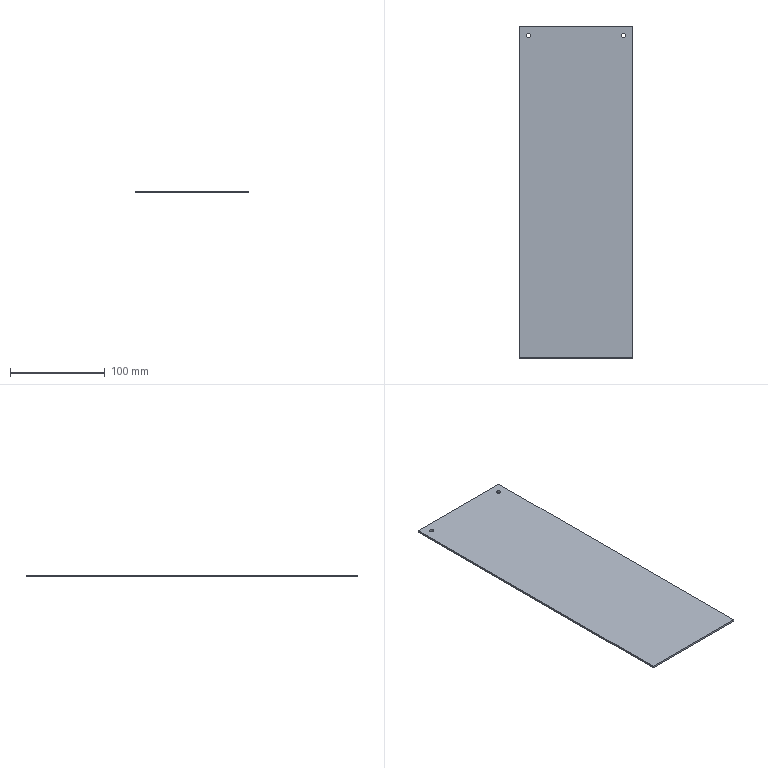Part | SolidWorks | features Extrusion 1, ICE 1 | 1 solid | 10 faces | box 120 x 350 x 2 mm | volume 83936 mm3 | plane 6 | cylinder 4 | commonest cylinder face diameters 4.5 x4
STEP:
#1=CARTESIAN_POINT('',(47.75,165.,0.));
#2=VERTEX_POINT('',#1);
#3=CARTESIAN_POINT('',(52.25,165.,0.));
#4=VERTEX_POINT('',#3);
#5=CARTESIAN_POINT('',(50.,165.,0.));
#6=DIRECTION('',(0.,0.,1.));
#7=DIRECTION('',(1.,0.,0.));
#8=AXIS2_PLACEMENT_3D('',#5,#6,#7);
#9=CIRCLE('',#8,2.25);
#10=EDGE_CURVE('',#2,#4,#9,.T.);
#11=ORIENTED_EDGE('',*,*,#10,.F.);
#12=CARTESIAN_POINT('',(47.75,165.,2.));
#13=VERTEX_POINT('',#12);
#14=CARTESIAN_POINT('',(47.75,165.,-8.));
#15=DIRECTION('',(0.,0.,1.));
#16=VECTOR('',#15,1000.);
#17=LINE('',#14,#16);
#18=EDGE_CURVE('',#2,#13,#17,.T.);
#19=ORIENTED_EDGE('',*,*,#18,.T.);
#20=CARTESIAN_POINT('',(52.25,165.,2.));
#21=VERTEX_POINT('',#20);
#22=CARTESIAN_POINT('',(50.,165.,2.));
#23=DIRECTION('',(0.,0.,1.));
#24=DIRECTION('',(1.,0.,0.));
#25=AXIS2_PLACEMENT_3D('',#22,#23,#24);
#26=CIRCLE('',#25,2.25);
#27=EDGE_CURVE('',#13,#21,#26,.T.);
#28=ORIENTED_EDGE('',*,*,#27,.T.);
#29=CARTESIAN_POINT('',(52.25,165.,-8.));
#30=DIRECTION('',(0.,0.,1.));
#31=VECTOR('',#30,1000.);
#32=LINE('',#29,#31);
#33=EDGE_CURVE('',#4,#21,#32,.T.);
#34=ORIENTED_EDGE('',*,*,#33,.F.);
#35=EDGE_LOOP('',(#11,#19,#28,#34));
#36=FACE_OUTER_BOUND('',#35,.T.);
#37=CARTESIAN_POINT('',(50.,165.,-8.));
#38=DIRECTION('',(0.,0.,1.));
#39=DIRECTION('',(1.,0.,0.));
#40=AXIS2_PLACEMENT_3D('',#37,#38,#39);
#41=CYLINDRICAL_SURFACE('',#40,2.25);
#42=ADVANCED_FACE('',(#36),#41,.F.);
#43=CARTESIAN_POINT('',(-52.25,165.,0.));
#44=VERTEX_POINT('',#43);
#45=CARTESIAN_POINT('',(-47.75,165.,0.));
#46=VERTEX_POINT('',#45);
#47=CARTESIAN_POINT('',(-50.,165.,0.));
#48=DIRECTION('',(0.,0.,1.));
#49=DIRECTION('',(1.,0.,0.));
#50=AXIS2_PLACEMENT_3D('',#47,#48,#49);
#51=CIRCLE('',#50,2.25);
#52=EDGE_CURVE('',#44,#46,#51,.T.);
#53=ORIENTED_EDGE('',*,*,#52,.F.);
#54=CARTESIAN_POINT('',(-52.25,165.,2.));
#55=VERTEX_POINT('',#54);
#56=CARTESIAN_POINT('',(-52.25,165.,-8.));
#57=DIRECTION('',(0.,0.,1.));
#58=VECTOR('',#57,1000.);
#59=LINE('',#56,#58);
#60=EDGE_CURVE('',#44,#55,#59,.T.);
#61=ORIENTED_EDGE('',*,*,#60,.T.);
#62=CARTESIAN_POINT('',(-47.75,165.,2.));
#63=VERTEX_POINT('',#62);
#64=CARTESIAN_POINT('',(-50.,165.,2.));
#65=DIRECTION('',(0.,0.,1.));
#66=DIRECTION('',(1.,0.,0.));
#67=AXIS2_PLACEMENT_3D('',#64,#65,#66);
#68=CIRCLE('',#67,2.25);
#69=EDGE_CURVE('',#55,#63,#68,.T.);
#70=ORIENTED_EDGE('',*,*,#69,.T.);
#71=CARTESIAN_POINT('',(-47.75,165.,-8.));
#72=DIRECTION('',(0.,0.,1.));
#73=VECTOR('',#72,1000.);
#74=LINE('',#71,#73);
#75=EDGE_CURVE('',#46,#63,#74,.T.);
#76=ORIENTED_EDGE('',*,*,#75,.F.);
#77=EDGE_LOOP('',(#53,#61,#70,#76));
#78=FACE_OUTER_BOUND('',#77,.T.);
#79=CARTESIAN_POINT('',(-50.,165.,-8.));
#80=DIRECTION('',(0.,0.,1.));
#81=DIRECTION('',(1.,0.,0.));
#82=AXIS2_PLACEMENT_3D('',#79,#80,#81);
#83=CYLINDRICAL_SURFACE('',#82,2.25);
#84=ADVANCED_FACE('',(#78),#83,.F.);
#85=CARTESIAN_POINT('',(60.,-175.,0.));
#86=VERTEX_POINT('',#85);
#87=CARTESIAN_POINT('',(60.,175.,0.));
#88=VERTEX_POINT('',#87);
#89=CARTESIAN_POINT('',(60.,175.,0.));
#90=DIRECTION('',(0.,1.,0.));
#91=VECTOR('',#90,1000.);
#92=LINE('',#89,#91);
#93=EDGE_CURVE('',#86,#88,#92,.T.);
#94=ORIENTED_EDGE('',*,*,#93,.T.);
#95=CARTESIAN_POINT('',(60.,175.,2.));
#96=VERTEX_POINT('',#95);
#97=CARTESIAN_POINT('',(60.,175.,2.));
#98=DIRECTION('',(0.,0.,-1.));
#99=VECTOR('',#98,1000.);
#100=LINE('',#97,#99);
#101=EDGE_CURVE('',#96,#88,#100,.T.);
#102=ORIENTED_EDGE('',*,*,#101,.F.);
#103=CARTESIAN_POINT('',(60.,-175.,2.));
#104=VERTEX_POINT('',#103);
#105=CARTESIAN_POINT('',(60.,175.,2.));
#106=DIRECTION('',(0.,1.,0.));
#107=VECTOR('',#106,1000.);
#108=LINE('',#105,#107);
#109=EDGE_CURVE('',#104,#96,#108,.T.);
#110=ORIENTED_EDGE('',*,*,#109,.F.);
#111=CARTESIAN_POINT('',(60.,-175.,2.));
#112=DIRECTION('',(0.,0.,-1.));
#113=VECTOR('',#112,1000.);
#114=LINE('',#111,#113);
#115=EDGE_CURVE('',#104,#86,#114,.T.);
#116=ORIENTED_EDGE('',*,*,#115,.T.);
#117=EDGE_LOOP('',(#94,#102,#110,#116));
#118=FACE_OUTER_BOUND('',#117,.T.);
#119=CARTESIAN_POINT('',(60.,175.,2.));
#120=DIRECTION('',(-1.,0.,0.));
#121=DIRECTION('',(0.,0.,1.));
#122=AXIS2_PLACEMENT_3D('',#119,#120,#121);
#123=PLANE('',#122);
#124=ADVANCED_FACE('',(#118),#123,.F.);
#125=CARTESIAN_POINT('',(-60.,175.,0.));
#126=VERTEX_POINT('',#125);
#127=CARTESIAN_POINT('',(-60.,175.,0.));
#128=DIRECTION('',(-1.,0.,0.));
#129=VECTOR('',#128,1000.);
#130=LINE('',#127,#129);
#131=EDGE_CURVE('',#88,#126,#130,.T.);
#132=ORIENTED_EDGE('',*,*,#131,.T.);
#133=CARTESIAN_POINT('',(-60.,175.,2.));
#134=VERTEX_POINT('',#133);
#135=CARTESIAN_POINT('',(-60.,175.,2.));
#136=DIRECTION('',(0.,0.,-1.));
#137=VECTOR('',#136,1000.);
#138=LINE('',#135,#137);
#139=EDGE_CURVE('',#134,#126,#138,.T.);
#140=ORIENTED_EDGE('',*,*,#139,.F.);
#141=CARTESIAN_POINT('',(-60.,175.,2.));
#142=DIRECTION('',(-1.,0.,0.));
#143=VECTOR('',#142,1000.);
#144=LINE('',#141,#143);
#145=EDGE_CURVE('',#96,#134,#144,.T.);
#146=ORIENTED_EDGE('',*,*,#145,.F.);
#147=ORIENTED_EDGE('',*,*,#101,.T.);
#148=EDGE_LOOP('',(#132,#140,#146,#147));
#149=FACE_OUTER_BOUND('',#148,.T.);
#150=CARTESIAN_POINT('',(-60.,175.,2.));
#151=DIRECTION('',(0.,-1.,0.));
#152=DIRECTION('',(0.,0.,-1.));
#153=AXIS2_PLACEMENT_3D('',#150,#151,#152);
#154=PLANE('',#153);
#155=ADVANCED_FACE('',(#149),#154,.F.);
#156=CARTESIAN_POINT('',(-60.,-175.,0.));
#157=VERTEX_POINT('',#156);
#158=CARTESIAN_POINT('',(-60.,175.,0.));
#159=DIRECTION('',(0.,-1.,0.));
#160=VECTOR('',#159,1000.);
#161=LINE('',#158,#160);
#162=EDGE_CURVE('',#126,#157,#161,.T.);
#163=ORIENTED_EDGE('',*,*,#162,.T.);
#164=CARTESIAN_POINT('',(-60.,-175.,2.));
#165=VERTEX_POINT('',#164);
#166=CARTESIAN_POINT('',(-60.,-175.,2.));
#167=DIRECTION('',(0.,0.,-1.));
#168=VECTOR('',#167,1000.);
#169=LINE('',#166,#168);
#170=EDGE_CURVE('',#165,#157,#169,.T.);
#171=ORIENTED_EDGE('',*,*,#170,.F.);
#172=CARTESIAN_POINT('',(-60.,175.,2.));
#173=DIRECTION('',(0.,-1.,0.));
#174=VECTOR('',#173,1000.);
#175=LINE('',#172,#174);
#176=EDGE_CURVE('',#134,#165,#175,.T.);
#177=ORIENTED_EDGE('',*,*,#176,.F.);
#178=ORIENTED_EDGE('',*,*,#139,.T.);
#179=EDGE_LOOP('',(#163,#171,#177,#178));
#180=FACE_OUTER_BOUND('',#179,.T.);
#181=CARTESIAN_POINT('',(-60.,175.,2.));
#182=DIRECTION('',(1.,0.,0.));
#183=DIRECTION('',(0.,0.,-1.));
#184=AXIS2_PLACEMENT_3D('',#181,#182,#183);
#185=PLANE('',#184);
#186=ADVANCED_FACE('',(#180),#185,.F.);
#187=CARTESIAN_POINT('',(-60.,-175.,0.));
#188=DIRECTION('',(1.,0.,0.));
#189=VECTOR('',#188,1000.);
#190=LINE('',#187,#189);
#191=EDGE_CURVE('',#157,#86,#190,.T.);
#192=ORIENTED_EDGE('',*,*,#191,.T.);
#193=ORIENTED_EDGE('',*,*,#115,.F.);
#194=CARTESIAN_POINT('',(-60.,-175.,2.));
#195=DIRECTION('',(1.,0.,0.));
#196=VECTOR('',#195,1000.);
#197=LINE('',#194,#196);
#198=EDGE_CURVE('',#165,#104,#197,.T.);
#199=ORIENTED_EDGE('',*,*,#198,.F.);
#200=ORIENTED_EDGE('',*,*,#170,.T.);
#201=EDGE_LOOP('',(#192,#193,#199,#200));
#202=FACE_OUTER_BOUND('',#201,.T.);
#203=CARTESIAN_POINT('',(-60.,-175.,2.));
#204=DIRECTION('',(0.,1.,0.));
#205=DIRECTION('',(0.,0.,1.));
#206=AXIS2_PLACEMENT_3D('',#203,#204,#205);
#207=PLANE('',#206);
#208=ADVANCED_FACE('',(#202),#207,.F.);
#209=CARTESIAN_POINT('',(50.,165.,2.));
#210=DIRECTION('',(0.,0.,1.));
#211=DIRECTION('',(1.,0.,0.));
#212=AXIS2_PLACEMENT_3D('',#209,#210,#211);
#213=CIRCLE('',#212,2.25);
#214=EDGE_CURVE('',#21,#13,#213,.T.);
#215=ORIENTED_EDGE('',*,*,#214,.F.);
#216=ORIENTED_EDGE('',*,*,#27,.F.);
#217=EDGE_LOOP('',(#215,#216));
#218=FACE_BOUND('',#217,.T.);
#219=CARTESIAN_POINT('',(-50.,165.,2.));
#220=DIRECTION('',(0.,0.,1.));
#221=DIRECTION('',(1.,0.,0.));
#222=AXIS2_PLACEMENT_3D('',#219,#220,#221);
#223=CIRCLE('',#222,2.25);
#224=EDGE_CURVE('',#63,#55,#223,.T.);
#225=ORIENTED_EDGE('',*,*,#224,.F.);
#226=ORIENTED_EDGE('',*,*,#69,.F.);
#227=EDGE_LOOP('',(#225,#226));
#228=FACE_BOUND('',#227,.T.);
#229=ORIENTED_EDGE('',*,*,#109,.T.);
#230=ORIENTED_EDGE('',*,*,#145,.T.);
#231=ORIENTED_EDGE('',*,*,#176,.T.);
#232=ORIENTED_EDGE('',*,*,#198,.T.);
#233=EDGE_LOOP('',(#229,#230,#231,#232));
#234=FACE_OUTER_BOUND('',#233,.T.);
#235=CARTESIAN_POINT('',(0.,0.,2.));
#236=DIRECTION('',(0.,0.,1.));
#237=DIRECTION('',(1.,0.,0.));
#238=AXIS2_PLACEMENT_3D('',#235,#236,#237);
#239=PLANE('',#238);
#240=ADVANCED_FACE('',(#218,#228,#234),#239,.T.);
#241=CARTESIAN_POINT('',(50.,165.,0.));
#242=DIRECTION('',(0.,0.,1.));
#243=DIRECTION('',(1.,0.,0.));
#244=AXIS2_PLACEMENT_3D('',#241,#242,#243);
#245=CIRCLE('',#244,2.25);
#246=EDGE_CURVE('',#4,#2,#245,.T.);
#247=ORIENTED_EDGE('',*,*,#246,.T.);
#248=ORIENTED_EDGE('',*,*,#10,.T.);
#249=EDGE_LOOP('',(#247,#248));
#250=FACE_BOUND('',#249,.T.);
#251=CARTESIAN_POINT('',(-50.,165.,0.));
#252=DIRECTION('',(0.,0.,1.));
#253=DIRECTION('',(1.,0.,0.));
#254=AXIS2_PLACEMENT_3D('',#251,#252,#253);
#255=CIRCLE('',#254,2.25);
#256=EDGE_CURVE('',#46,#44,#255,.T.);
#257=ORIENTED_EDGE('',*,*,#256,.T.);
#258=ORIENTED_EDGE('',*,*,#52,.T.);
#259=EDGE_LOOP('',(#257,#258));
#260=FACE_BOUND('',#259,.T.);
#261=ORIENTED_EDGE('',*,*,#93,.F.);
#262=ORIENTED_EDGE('',*,*,#191,.F.);
#263=ORIENTED_EDGE('',*,*,#162,.F.);
#264=ORIENTED_EDGE('',*,*,#131,.F.);
#265=EDGE_LOOP('',(#261,#262,#263,#264));
#266=FACE_OUTER_BOUND('',#265,.T.);
#267=CARTESIAN_POINT('',(0.,0.,0.));
#268=DIRECTION('',(0.,0.,1.));
#269=DIRECTION('',(1.,0.,0.));
#270=AXIS2_PLACEMENT_3D('',#267,#268,#269);
#271=PLANE('',#270);
#272=ADVANCED_FACE('',(#250,#260,#266),#271,.F.);
#273=ORIENTED_EDGE('',*,*,#60,.F.);
#274=ORIENTED_EDGE('',*,*,#256,.F.);
#275=ORIENTED_EDGE('',*,*,#75,.T.);
#276=ORIENTED_EDGE('',*,*,#224,.T.);
#277=EDGE_LOOP('',(#273,#274,#275,#276));
#278=FACE_OUTER_BOUND('',#277,.T.);
#279=CARTESIAN_POINT('',(-50.,165.,-8.));
#280=DIRECTION('',(0.,0.,1.));
#281=DIRECTION('',(1.,0.,0.));
#282=AXIS2_PLACEMENT_3D('',#279,#280,#281);
#283=CYLINDRICAL_SURFACE('',#282,2.25);
#284=ADVANCED_FACE('',(#278),#283,.F.);
#285=ORIENTED_EDGE('',*,*,#18,.F.);
#286=ORIENTED_EDGE('',*,*,#246,.F.);
#287=ORIENTED_EDGE('',*,*,#33,.T.);
#288=ORIENTED_EDGE('',*,*,#214,.T.);
#289=EDGE_LOOP('',(#285,#286,#287,#288));
#290=FACE_OUTER_BOUND('',#289,.T.);
#291=CARTESIAN_POINT('',(50.,165.,-8.));
#292=DIRECTION('',(0.,0.,1.));
#293=DIRECTION('',(1.,0.,0.));
#294=AXIS2_PLACEMENT_3D('',#291,#292,#293);
#295=CYLINDRICAL_SURFACE('',#294,2.25);
#296=ADVANCED_FACE('',(#290),#295,.F.);
#297=CLOSED_SHELL('',(#42,#84,#124,#155,#186,#208,#240,#272,#284,#296));
#298=MANIFOLD_SOLID_BREP('',#297);
#299=CARTESIAN_POINT('',(0.,0.,0.));
#300=DIRECTION('',(0.,0.,1.));
#301=DIRECTION('',(1.,0.,0.));
#302=AXIS2_PLACEMENT_3D('',#299,#300,#301);
#303=(LENGTH_UNIT()NAMED_UNIT(*)SI_UNIT(.MILLI.,.METRE.));
#304=UNCERTAINTY_MEASURE_WITH_UNIT(LENGTH_MEASURE(0.00001),#303,'','');
#305=(NAMED_UNIT(*)PLANE_ANGLE_UNIT()SI_UNIT($,.RADIAN.));
#306=(NAMED_UNIT(*)SI_UNIT($,.STERADIAN.)SOLID_ANGLE_UNIT());
#307=(GEOMETRIC_REPRESENTATION_CONTEXT(3)GLOBAL_UNCERTAINTY_ASSIGNED_CONTEXT((#304))GLOBAL_UNIT_ASSIGNED_CONTEXT((#303,#305,#306))REPRESENTATION_CONTEXT('',''));
#308=ADVANCED_BREP_SHAPE_REPRESENTATION('',(#298,#302),#307);